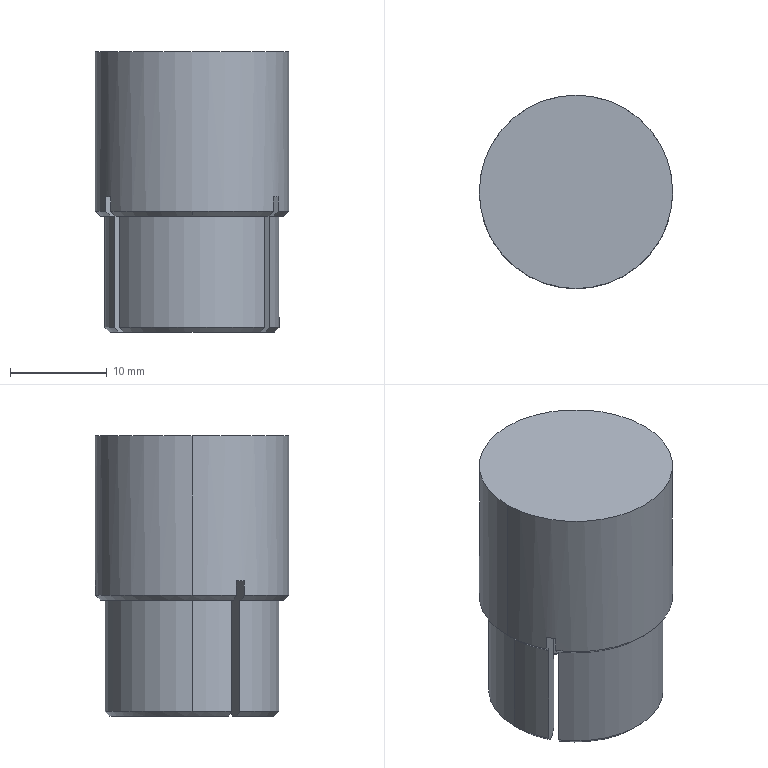Part | STEP file | BABR060_X2_8f9351658f74_X0_-14.STEP | 1 solid | 40 faces | box 20 x 20 x 29 mm | volume 3932 mm3 | plane 18 | cone 12 | cylinder 10 | commonest cylinder face diameters 18 x4 14 x2 15 x2 20 x2
STEP:
#1=CARTESIAN_POINT('',(-10.,0.,29.));
#2=VERTEX_POINT('',#1);
#3=CARTESIAN_POINT('',(10.,0.,29.));
#4=VERTEX_POINT('',#3);
#5=CARTESIAN_POINT('',(0.,0.,29.));
#6=DIRECTION('',(0.,0.,-1.));
#7=DIRECTION('',(-1.,0.,0.));
#8=AXIS2_PLACEMENT_3D('',#5,#6,#7);
#9=CIRCLE('',#8,10.);
#10=EDGE_CURVE('',#2,#4,#9,.T.);
#11=ORIENTED_EDGE('',*,*,#10,.T.);
#12=CARTESIAN_POINT('',(10.,0.,12.5));
#13=VERTEX_POINT('',#12);
#14=CARTESIAN_POINT('',(10.,0.,29.));
#15=DIRECTION('',(0.,0.,-1.));
#16=VECTOR('',#15,1000.);
#17=LINE('',#14,#16);
#18=EDGE_CURVE('',#4,#13,#17,.T.);
#19=ORIENTED_EDGE('',*,*,#18,.T.);
#20=CARTESIAN_POINT('',(0.5,9.987,12.5));
#21=VERTEX_POINT('',#20);
#22=CARTESIAN_POINT('',(0.,0.,12.5));
#23=DIRECTION('',(0.,0.,1.));
#24=DIRECTION('',(-1.,0.,0.));
#25=AXIS2_PLACEMENT_3D('',#22,#23,#24);
#26=CIRCLE('',#25,10.);
#27=EDGE_CURVE('',#13,#21,#26,.T.);
#28=ORIENTED_EDGE('',*,*,#27,.T.);
#29=CARTESIAN_POINT('',(0.5,9.987,14.));
#30=VERTEX_POINT('',#29);
#31=CARTESIAN_POINT('',(0.5,9.987,14.));
#32=DIRECTION('',(0.,0.,1.));
#33=VECTOR('',#32,1000.);
#34=LINE('',#31,#33);
#35=EDGE_CURVE('',#21,#30,#34,.T.);
#36=ORIENTED_EDGE('',*,*,#35,.T.);
#37=CARTESIAN_POINT('',(-0.5,9.987,14.));
#38=VERTEX_POINT('',#37);
#39=CARTESIAN_POINT('',(0.,0.,14.));
#40=DIRECTION('',(0.,0.,1.));
#41=DIRECTION('',(-1.,0.,0.));
#42=AXIS2_PLACEMENT_3D('',#39,#40,#41);
#43=CIRCLE('',#42,10.);
#44=EDGE_CURVE('',#30,#38,#43,.T.);
#45=ORIENTED_EDGE('',*,*,#44,.T.);
#46=CARTESIAN_POINT('',(-0.5,9.987,12.5));
#47=VERTEX_POINT('',#46);
#48=CARTESIAN_POINT('',(-0.5,9.987,14.));
#49=DIRECTION('',(0.,0.,-1.));
#50=VECTOR('',#49,1000.);
#51=LINE('',#48,#50);
#52=EDGE_CURVE('',#38,#47,#51,.T.);
#53=ORIENTED_EDGE('',*,*,#52,.T.);
#54=CARTESIAN_POINT('',(-10.,0.,12.5));
#55=VERTEX_POINT('',#54);
#56=CARTESIAN_POINT('',(0.,0.,12.5));
#57=DIRECTION('',(0.,0.,1.));
#58=DIRECTION('',(-1.,0.,0.));
#59=AXIS2_PLACEMENT_3D('',#56,#57,#58);
#60=CIRCLE('',#59,10.);
#61=EDGE_CURVE('',#47,#55,#60,.T.);
#62=ORIENTED_EDGE('',*,*,#61,.T.);
#63=CARTESIAN_POINT('',(-10.,0.,29.));
#64=DIRECTION('',(0.,0.,-1.));
#65=VECTOR('',#64,1000.);
#66=LINE('',#63,#65);
#67=EDGE_CURVE('',#2,#55,#66,.T.);
#68=ORIENTED_EDGE('',*,*,#67,.F.);
#69=EDGE_LOOP('',(#11,#19,#28,#36,#45,#53,#62,#68));
#70=FACE_OUTER_BOUND('',#69,.T.);
#71=CARTESIAN_POINT('',(0.,0.,29.));
#72=DIRECTION('',(0.,0.,-1.));
#73=DIRECTION('',(-1.,0.,0.));
#74=AXIS2_PLACEMENT_3D('',#71,#72,#73);
#75=CYLINDRICAL_SURFACE('',#74,10.);
#76=ADVANCED_FACE('',(#70),#75,.T.);
#77=CARTESIAN_POINT('',(-7.966,-5.176,12.));
#78=VERTEX_POINT('',#77);
#79=CARTESIAN_POINT('',(0.,-9.5,12.));
#80=VERTEX_POINT('',#79);
#81=CARTESIAN_POINT('',(0.,0.,12.));
#82=DIRECTION('',(0.,0.,1.));
#83=DIRECTION('',(0.,-1.,0.));
#84=AXIS2_PLACEMENT_3D('',#81,#82,#83);
#85=CIRCLE('',#84,9.5);
#86=EDGE_CURVE('',#78,#80,#85,.T.);
#87=ORIENTED_EDGE('',*,*,#86,.T.);
#88=CARTESIAN_POINT('',(0.,-10.,12.5));
#89=VERTEX_POINT('',#88);
#90=CARTESIAN_POINT('',(0.,-10.,12.5));
#91=DIRECTION('',(0.,-0.7071,0.7071));
#92=VECTOR('',#91,1000.);
#93=LINE('',#90,#92);
#94=EDGE_CURVE('',#80,#89,#93,.T.);
#95=ORIENTED_EDGE('',*,*,#94,.T.);
#96=CARTESIAN_POINT('',(-8.399,-5.427,12.5));
#97=VERTEX_POINT('',#96);
#98=CARTESIAN_POINT('',(0.,0.,12.5));
#99=DIRECTION('',(0.,0.,1.));
#100=DIRECTION('',(-1.,0.,0.));
#101=AXIS2_PLACEMENT_3D('',#98,#99,#100);
#102=CIRCLE('',#101,10.);
#103=EDGE_CURVE('',#97,#89,#102,.T.);
#104=ORIENTED_EDGE('',*,*,#103,.F.);
#105=CARTESIAN_POINT('',(-8.399,-5.427,12.5));
#106=CARTESIAN_POINT('',(-8.255,-5.343,12.333));
#107=CARTESIAN_POINT('',(-8.11,-5.26,12.167));
#108=CARTESIAN_POINT('',(-7.966,-5.176,12.));
#109=B_SPLINE_CURVE_WITH_KNOTS('',3,(#105,#106,#107,#108),.UNSPECIFIED.,.F.,.F.,(4,4),(0.,0.0007076),.UNSPECIFIED.);
#110=EDGE_CURVE('',#97,#78,#109,.T.);
#111=ORIENTED_EDGE('',*,*,#110,.T.);
#112=EDGE_LOOP('',(#87,#95,#104,#111));
#113=FACE_OUTER_BOUND('',#112,.T.);
#114=CARTESIAN_POINT('',(0.,0.,12.5));
#115=DIRECTION('',(0.,0.,1.));
#116=DIRECTION('',(0.,-1.,0.));
#117=AXIS2_PLACEMENT_3D('',#114,#115,#116);
#118=CONICAL_SURFACE('',#117,10.,0.7854);
#119=ADVANCED_FACE('',(#113),#118,.T.);
#120=CARTESIAN_POINT('',(-8.032,-4.06,12.));
#121=VERTEX_POINT('',#120);
#122=CARTESIAN_POINT('',(-9.,0.,12.));
#123=VERTEX_POINT('',#122);
#124=CARTESIAN_POINT('',(0.,0.,12.));
#125=DIRECTION('',(0.,0.,-1.));
#126=DIRECTION('',(-1.,0.,0.));
#127=AXIS2_PLACEMENT_3D('',#124,#125,#126);
#128=CIRCLE('',#127,9.);
#129=EDGE_CURVE('',#121,#123,#128,.T.);
#130=ORIENTED_EDGE('',*,*,#129,.T.);
#131=CARTESIAN_POINT('',(-9.,0.,0.5));
#132=VERTEX_POINT('',#131);
#133=CARTESIAN_POINT('',(-9.,0.,12.));
#134=DIRECTION('',(0.,0.,-1.));
#135=VECTOR('',#134,1000.);
#136=LINE('',#133,#135);
#137=EDGE_CURVE('',#123,#132,#136,.T.);
#138=ORIENTED_EDGE('',*,*,#137,.T.);
#139=CARTESIAN_POINT('',(-8.032,-4.06,0.5));
#140=VERTEX_POINT('',#139);
#141=CARTESIAN_POINT('',(0.,0.,0.5));
#142=DIRECTION('',(0.,0.,1.));
#143=DIRECTION('',(-1.,0.,0.));
#144=AXIS2_PLACEMENT_3D('',#141,#142,#143);
#145=CIRCLE('',#144,9.);
#146=EDGE_CURVE('',#132,#140,#145,.T.);
#147=ORIENTED_EDGE('',*,*,#146,.T.);
#148=CARTESIAN_POINT('',(-8.032,-4.06,12.));
#149=DIRECTION('',(0.,0.,1.));
#150=VECTOR('',#149,1000.);
#151=LINE('',#148,#150);
#152=EDGE_CURVE('',#140,#121,#151,.T.);
#153=ORIENTED_EDGE('',*,*,#152,.T.);
#154=EDGE_LOOP('',(#130,#138,#147,#153));
#155=FACE_OUTER_BOUND('',#154,.T.);
#156=CARTESIAN_POINT('',(0.,0.,12.));
#157=DIRECTION('',(0.,0.,-1.));
#158=DIRECTION('',(-1.,0.,0.));
#159=AXIS2_PLACEMENT_3D('',#156,#157,#158);
#160=CYLINDRICAL_SURFACE('',#159,9.);
#161=ADVANCED_FACE('',(#155),#160,.T.);
#162=CARTESIAN_POINT('',(7.598,-3.81,0.));
#163=VERTEX_POINT('',#162);
#164=CARTESIAN_POINT('',(8.5,0.,0.));
#165=VERTEX_POINT('',#164);
#166=CARTESIAN_POINT('',(0.,0.,0.));
#167=DIRECTION('',(0.,0.,1.));
#168=DIRECTION('',(1.,0.,0.));
#169=AXIS2_PLACEMENT_3D('',#166,#167,#168);
#170=CIRCLE('',#169,8.5);
#171=EDGE_CURVE('',#163,#165,#170,.T.);
#172=ORIENTED_EDGE('',*,*,#171,.T.);
#173=CARTESIAN_POINT('',(9.,0.,0.5));
#174=VERTEX_POINT('',#173);
#175=CARTESIAN_POINT('',(9.,0.,0.5));
#176=DIRECTION('',(0.7071,0.,0.7071));
#177=VECTOR('',#176,1000.);
#178=LINE('',#175,#177);
#179=EDGE_CURVE('',#165,#174,#178,.T.);
#180=ORIENTED_EDGE('',*,*,#179,.T.);
#181=CARTESIAN_POINT('',(8.032,-4.06,0.5));
#182=VERTEX_POINT('',#181);
#183=CARTESIAN_POINT('',(0.,0.,0.5));
#184=DIRECTION('',(0.,0.,1.));
#185=DIRECTION('',(-1.,0.,0.));
#186=AXIS2_PLACEMENT_3D('',#183,#184,#185);
#187=CIRCLE('',#186,9.);
#188=EDGE_CURVE('',#182,#174,#187,.T.);
#189=ORIENTED_EDGE('',*,*,#188,.F.);
#190=CARTESIAN_POINT('',(8.032,-4.06,0.5));
#191=CARTESIAN_POINT('',(7.888,-3.977,0.3333));
#192=CARTESIAN_POINT('',(7.743,-3.893,0.1667));
#193=CARTESIAN_POINT('',(7.598,-3.81,0.));
#194=B_SPLINE_CURVE_WITH_KNOTS('',3,(#190,#191,#192,#193),.UNSPECIFIED.,.F.,.F.,(4,4),(0.,0.0007077),.UNSPECIFIED.);
#195=EDGE_CURVE('',#182,#163,#194,.T.);
#196=ORIENTED_EDGE('',*,*,#195,.T.);
#197=EDGE_LOOP('',(#172,#180,#189,#196));
#198=FACE_OUTER_BOUND('',#197,.T.);
#199=CARTESIAN_POINT('',(0.,0.,0.5));
#200=DIRECTION('',(0.,0.,1.));
#201=DIRECTION('',(1.,0.,0.));
#202=AXIS2_PLACEMENT_3D('',#199,#200,#201);
#203=CONICAL_SURFACE('',#202,9.,0.7854);
#204=ADVANCED_FACE('',(#198),#203,.T.);
#205=CARTESIAN_POINT('',(7.,0.,14.5));
#206=VERTEX_POINT('',#205);
#207=CARTESIAN_POINT('',(-7.,0.,14.5));
#208=VERTEX_POINT('',#207);
#209=CARTESIAN_POINT('',(0.,0.,14.5));
#210=DIRECTION('',(0.,0.,-1.));
#211=DIRECTION('',(-1.,0.,0.));
#212=AXIS2_PLACEMENT_3D('',#209,#210,#211);
#213=CIRCLE('',#212,7.);
#214=EDGE_CURVE('',#206,#208,#213,.T.);
#215=ORIENTED_EDGE('',*,*,#214,.F.);
#216=CARTESIAN_POINT('',(7.,0.,0.5));
#217=VERTEX_POINT('',#216);
#218=CARTESIAN_POINT('',(7.,0.,14.5));
#219=DIRECTION('',(0.,0.,-1.));
#220=VECTOR('',#219,1000.);
#221=LINE('',#218,#220);
#222=EDGE_CURVE('',#206,#217,#221,.T.);
#223=ORIENTED_EDGE('',*,*,#222,.T.);
#224=CARTESIAN_POINT('',(6.297,-3.058,0.5));
#225=VERTEX_POINT('',#224);
#226=CARTESIAN_POINT('',(0.,0.,0.5));
#227=DIRECTION('',(0.,0.,1.));
#228=DIRECTION('',(-1.,0.,0.));
#229=AXIS2_PLACEMENT_3D('',#226,#227,#228);
#230=CIRCLE('',#229,7.);
#231=EDGE_CURVE('',#225,#217,#230,.T.);
#232=ORIENTED_EDGE('',*,*,#231,.F.);
#233=CARTESIAN_POINT('',(6.297,-3.058,14.));
#234=VERTEX_POINT('',#233);
#235=CARTESIAN_POINT('',(6.297,-3.058,14.));
#236=DIRECTION('',(0.,0.,1.));
#237=VECTOR('',#236,1000.);
#238=LINE('',#235,#237);
#239=EDGE_CURVE('',#225,#234,#238,.T.);
#240=ORIENTED_EDGE('',*,*,#239,.T.);
#241=CARTESIAN_POINT('',(5.797,-3.924,14.));
#242=VERTEX_POINT('',#241);
#243=CARTESIAN_POINT('',(0.,0.,14.));
#244=DIRECTION('',(0.,0.,1.));
#245=DIRECTION('',(-1.,0.,0.));
#246=AXIS2_PLACEMENT_3D('',#243,#244,#245);
#247=CIRCLE('',#246,7.);
#248=EDGE_CURVE('',#242,#234,#247,.T.);
#249=ORIENTED_EDGE('',*,*,#248,.F.);
#250=CARTESIAN_POINT('',(5.797,-3.924,0.5));
#251=VERTEX_POINT('',#250);
#252=CARTESIAN_POINT('',(5.797,-3.924,14.));
#253=DIRECTION('',(0.,0.,-1.));
#254=VECTOR('',#253,1000.);
#255=LINE('',#252,#254);
#256=EDGE_CURVE('',#242,#251,#255,.T.);
#257=ORIENTED_EDGE('',*,*,#256,.T.);
#258=CARTESIAN_POINT('',(-5.797,-3.924,0.5));
#259=VERTEX_POINT('',#258);
#260=CARTESIAN_POINT('',(0.,0.,0.5));
#261=DIRECTION('',(0.,0.,1.));
#262=DIRECTION('',(-1.,0.,0.));
#263=AXIS2_PLACEMENT_3D('',#260,#261,#262);
#264=CIRCLE('',#263,7.);
#265=EDGE_CURVE('',#259,#251,#264,.T.);
#266=ORIENTED_EDGE('',*,*,#265,.F.);
#267=CARTESIAN_POINT('',(-5.797,-3.924,14.));
#268=VERTEX_POINT('',#267);
#269=CARTESIAN_POINT('',(-5.797,-3.924,14.));
#270=DIRECTION('',(0.,0.,1.));
#271=VECTOR('',#270,1000.);
#272=LINE('',#269,#271);
#273=EDGE_CURVE('',#259,#268,#272,.T.);
#274=ORIENTED_EDGE('',*,*,#273,.T.);
#275=CARTESIAN_POINT('',(-6.297,-3.058,14.));
#276=VERTEX_POINT('',#275);
#277=CARTESIAN_POINT('',(0.,0.,14.));
#278=DIRECTION('',(0.,0.,-1.));
#279=DIRECTION('',(-1.,0.,0.));
#280=AXIS2_PLACEMENT_3D('',#277,#278,#279);
#281=CIRCLE('',#280,7.);
#282=EDGE_CURVE('',#268,#276,#281,.T.);
#283=ORIENTED_EDGE('',*,*,#282,.T.);
#284=CARTESIAN_POINT('',(-6.297,-3.058,0.5));
#285=VERTEX_POINT('',#284);
#286=CARTESIAN_POINT('',(-6.297,-3.058,14.));
#287=DIRECTION('',(0.,0.,-1.));
#288=VECTOR('',#287,1000.);
#289=LINE('',#286,#288);
#290=EDGE_CURVE('',#276,#285,#289,.T.);
#291=ORIENTED_EDGE('',*,*,#290,.T.);
#292=CARTESIAN_POINT('',(-7.,0.,0.5));
#293=VERTEX_POINT('',#292);
#294=CARTESIAN_POINT('',(0.,0.,0.5));
#295=DIRECTION('',(0.,0.,1.));
#296=DIRECTION('',(-1.,0.,0.));
#297=AXIS2_PLACEMENT_3D('',#294,#295,#296);
#298=CIRCLE('',#297,7.);
#299=EDGE_CURVE('',#293,#285,#298,.T.);
#300=ORIENTED_EDGE('',*,*,#299,.F.);
#301=CARTESIAN_POINT('',(-7.,0.,14.5));
#302=DIRECTION('',(0.,0.,-1.));
#303=VECTOR('',#302,1000.);
#304=LINE('',#301,#303);
#305=EDGE_CURVE('',#208,#293,#304,.T.);
#306=ORIENTED_EDGE('',*,*,#305,.F.);
#307=EDGE_LOOP('',(#215,#223,#232,#240,#249,#257,#266,#274,#283,#291,#300,#306));
#308=FACE_OUTER_BOUND('',#307,.T.);
#309=CARTESIAN_POINT('',(0.,0.,14.5));
#310=DIRECTION('',(0.,0.,-1.));
#311=DIRECTION('',(-1.,0.,0.));
#312=AXIS2_PLACEMENT_3D('',#309,#310,#311);
#313=CYLINDRICAL_SURFACE('',#312,7.);
#314=ADVANCED_FACE('',(#308),#313,.F.);
#315=CARTESIAN_POINT('',(-0.5,6.982,0.5));
#316=VERTEX_POINT('',#315);
#317=CARTESIAN_POINT('',(0.,0.,0.5));
#318=DIRECTION('',(0.,0.,1.));
#319=DIRECTION('',(-1.,0.,0.));
#320=AXIS2_PLACEMENT_3D('',#317,#318,#319);
#321=CIRCLE('',#320,7.);
#322=EDGE_CURVE('',#316,#293,#321,.T.);
#323=ORIENTED_EDGE('',*,*,#322,.T.);
#324=CARTESIAN_POINT('',(-7.5,0.,0.));
#325=VERTEX_POINT('',#324);
#326=CARTESIAN_POINT('',(-7.5,0.,0.));
#327=DIRECTION('',(-0.7071,0.,-0.7071));
#328=VECTOR('',#327,1000.);
#329=LINE('',#326,#328);
#330=EDGE_CURVE('',#293,#325,#329,.T.);
#331=ORIENTED_EDGE('',*,*,#330,.T.);
#332=CARTESIAN_POINT('',(-0.5,7.483,0.));
#333=VERTEX_POINT('',#332);
#334=CARTESIAN_POINT('',(0.,0.,0.));
#335=DIRECTION('',(0.,0.,-1.));
#336=DIRECTION('',(-1.,0.,0.));
#337=AXIS2_PLACEMENT_3D('',#334,#335,#336);
#338=CIRCLE('',#337,7.5);
#339=EDGE_CURVE('',#325,#333,#338,.T.);
#340=ORIENTED_EDGE('',*,*,#339,.T.);
#341=CARTESIAN_POINT('',(-0.5,6.982,0.5));
#342=CARTESIAN_POINT('',(-0.5,7.149,0.3333));
#343=CARTESIAN_POINT('',(-0.5,7.316,0.1667));
#344=CARTESIAN_POINT('',(-0.5,7.483,0.));
#345=B_SPLINE_CURVE_WITH_KNOTS('',3,(#341,#342,#343,#344),.UNSPECIFIED.,.F.,.F.,(4,4),(0.,0.000708),.UNSPECIFIED.);
#346=EDGE_CURVE('',#316,#333,#345,.T.);
#347=ORIENTED_EDGE('',*,*,#346,.F.);
#348=EDGE_LOOP('',(#323,#331,#340,#347));
#349=FACE_OUTER_BOUND('',#348,.T.);
#350=CARTESIAN_POINT('',(0.,0.,0.));
#351=DIRECTION('',(0.,0.,-1.));
#352=DIRECTION('',(-1.,0.,0.));
#353=AXIS2_PLACEMENT_3D('',#350,#351,#352);
#354=CONICAL_SURFACE('',#353,7.5,0.7854);
#355=ADVANCED_FACE('',(#349),#354,.F.);
#356=CARTESIAN_POINT('',(7.5,0.,26.5));
#357=VERTEX_POINT('',#356);
#358=CARTESIAN_POINT('',(-7.5,0.,26.5));
#359=VERTEX_POINT('',#358);
#360=CARTESIAN_POINT('',(0.,0.,26.5));
#361=DIRECTION('',(0.,0.,-1.));
#362=DIRECTION('',(-1.,0.,0.));
#363=AXIS2_PLACEMENT_3D('',#360,#361,#362);
#364=CIRCLE('',#363,7.5);
#365=EDGE_CURVE('',#357,#359,#364,.T.);
#366=ORIENTED_EDGE('',*,*,#365,.F.);
#367=CARTESIAN_POINT('',(7.5,0.,14.5));
#368=VERTEX_POINT('',#367);
#369=CARTESIAN_POINT('',(7.5,0.,26.5));
#370=DIRECTION('',(0.,0.,-1.));
#371=VECTOR('',#370,1000.);
#372=LINE('',#369,#371);
#373=EDGE_CURVE('',#357,#368,#372,.T.);
#374=ORIENTED_EDGE('',*,*,#373,.T.);
#375=CARTESIAN_POINT('',(-7.5,0.,14.5));
#376=VERTEX_POINT('',#375);
#377=CARTESIAN_POINT('',(0.,0.,14.5));
#378=DIRECTION('',(0.,0.,-1.));
#379=DIRECTION('',(-1.,0.,0.));
#380=AXIS2_PLACEMENT_3D('',#377,#378,#379);
#381=CIRCLE('',#380,7.5);
#382=EDGE_CURVE('',#368,#376,#381,.T.);
#383=ORIENTED_EDGE('',*,*,#382,.T.);
#384=CARTESIAN_POINT('',(-7.5,0.,26.5));
#385=DIRECTION('',(0.,0.,-1.));
#386=VECTOR('',#385,1000.);
#387=LINE('',#384,#386);
#388=EDGE_CURVE('',#359,#376,#387,.T.);
#389=ORIENTED_EDGE('',*,*,#388,.F.);
#390=EDGE_LOOP('',(#366,#374,#383,#389));
#391=FACE_OUTER_BOUND('',#390,.T.);
#392=CARTESIAN_POINT('',(0.,0.,26.5));
#393=DIRECTION('',(0.,0.,-1.));
#394=DIRECTION('',(-1.,0.,0.));
#395=AXIS2_PLACEMENT_3D('',#392,#393,#394);
#396=CYLINDRICAL_SURFACE('',#395,7.5);
#397=ADVANCED_FACE('',(#391),#396,.F.);
#398=ORIENTED_EDGE('',*,*,#18,.F.);
#399=CARTESIAN_POINT('',(0.,0.,29.));
#400=DIRECTION('',(0.,0.,-1.));
#401=DIRECTION('',(-1.,0.,0.));
#402=AXIS2_PLACEMENT_3D('',#399,#400,#401);
#403=CIRCLE('',#402,10.);
#404=EDGE_CURVE('',#4,#2,#403,.T.);
#405=ORIENTED_EDGE('',*,*,#404,.T.);
#406=ORIENTED_EDGE('',*,*,#67,.T.);
#407=CARTESIAN_POINT('',(-8.899,-4.561,12.5));
#408=VERTEX_POINT('',#407);
#409=CARTESIAN_POINT('',(0.,0.,12.5));
#410=DIRECTION('',(0.,0.,1.));
#411=DIRECTION('',(-1.,0.,0.));
#412=AXIS2_PLACEMENT_3D('',#409,#410,#411);
#413=CIRCLE('',#412,10.);
#414=EDGE_CURVE('',#55,#408,#413,.T.);
#415=ORIENTED_EDGE('',*,*,#414,.T.);
#416=CARTESIAN_POINT('',(-8.899,-4.561,14.));
#417=VERTEX_POINT('',#416);
#418=CARTESIAN_POINT('',(-8.899,-4.561,14.));
#419=DIRECTION('',(0.,0.,1.));
#420=VECTOR('',#419,1000.);
#421=LINE('',#418,#420);
#422=EDGE_CURVE('',#408,#417,#421,.T.);
#423=ORIENTED_EDGE('',*,*,#422,.T.);
#424=CARTESIAN_POINT('',(-8.399,-5.427,14.));
#425=VERTEX_POINT('',#424);
#426=CARTESIAN_POINT('',(0.,0.,14.));
#427=DIRECTION('',(0.,0.,1.));
#428=DIRECTION('',(-1.,0.,0.));
#429=AXIS2_PLACEMENT_3D('',#426,#427,#428);
#430=CIRCLE('',#429,10.);
#431=EDGE_CURVE('',#417,#425,#430,.T.);
#432=ORIENTED_EDGE('',*,*,#431,.T.);
#433=CARTESIAN_POINT('',(-8.399,-5.427,14.));
#434=DIRECTION('',(0.,0.,-1.));
#435=VECTOR('',#434,1000.);
#436=LINE('',#433,#435);
#437=EDGE_CURVE('',#425,#97,#436,.T.);
#438=ORIENTED_EDGE('',*,*,#437,.T.);
#439=ORIENTED_EDGE('',*,*,#103,.T.);
#440=CARTESIAN_POINT('',(8.399,-5.427,12.5));
#441=VERTEX_POINT('',#440);
#442=CARTESIAN_POINT('',(0.,0.,12.5));
#443=DIRECTION('',(0.,0.,1.));
#444=DIRECTION('',(-1.,0.,0.));
#445=AXIS2_PLACEMENT_3D('',#442,#443,#444);
#446=CIRCLE('',#445,10.);
#447=EDGE_CURVE('',#89,#441,#446,.T.);
#448=ORIENTED_EDGE('',*,*,#447,.T.);
#449=CARTESIAN_POINT('',(8.399,-5.427,14.));
#450=VERTEX_POINT('',#449);
#451=CARTESIAN_POINT('',(8.399,-5.427,14.));
#452=DIRECTION('',(0.,0.,1.));
#453=VECTOR('',#452,1000.);
#454=LINE('',#451,#453);
#455=EDGE_CURVE('',#441,#450,#454,.T.);
#456=ORIENTED_EDGE('',*,*,#455,.T.);
#457=CARTESIAN_POINT('',(8.899,-4.561,14.));
#458=VERTEX_POINT('',#457);
#459=CARTESIAN_POINT('',(0.,0.,14.));
#460=DIRECTION('',(0.,0.,1.));
#461=DIRECTION('',(-1.,0.,0.));
#462=AXIS2_PLACEMENT_3D('',#459,#460,#461);
#463=CIRCLE('',#462,10.);
#464=EDGE_CURVE('',#450,#458,#463,.T.);
#465=ORIENTED_EDGE('',*,*,#464,.T.);
#466=CARTESIAN_POINT('',(8.899,-4.561,12.5));
#467=VERTEX_POINT('',#466);
#468=CARTESIAN_POINT('',(8.899,-4.561,14.));
#469=DIRECTION('',(0.,0.,-1.));
#470=VECTOR('',#469,1000.);
#471=LINE('',#468,#470);
#472=EDGE_CURVE('',#458,#467,#471,.T.);
#473=ORIENTED_EDGE('',*,*,#472,.T.);
#474=CARTESIAN_POINT('',(0.,0.,12.5));
#475=DIRECTION('',(0.,0.,1.));
#476=DIRECTION('',(-1.,0.,0.));
#477=AXIS2_PLACEMENT_3D('',#474,#475,#476);
#478=CIRCLE('',#477,10.);
#479=EDGE_CURVE('',#467,#13,#478,.T.);
#480=ORIENTED_EDGE('',*,*,#479,.T.);
#481=EDGE_LOOP('',(#398,#405,#406,#415,#423,#432,#438,#439,#448,#456,#465,#473,#480));
#482=FACE_OUTER_BOUND('',#481,.T.);
#483=CARTESIAN_POINT('',(0.,0.,29.));
#484=DIRECTION('',(0.,0.,-1.));
#485=DIRECTION('',(-1.,0.,0.));
#486=AXIS2_PLACEMENT_3D('',#483,#484,#485);
#487=CYLINDRICAL_SURFACE('',#486,10.);
#488=ADVANCED_FACE('',(#482),#487,.T.);
#489=CARTESIAN_POINT('',(-0.5,9.487,12.));
#490=VERTEX_POINT('',#489);
#491=CARTESIAN_POINT('',(-0.5,9.987,12.5));
#492=CARTESIAN_POINT('',(-0.5,9.821,12.333));
#493=CARTESIAN_POINT('',(-0.5,9.654,12.167));
#494=CARTESIAN_POINT('',(-0.5,9.487,12.));
#495=B_SPLINE_CURVE_WITH_KNOTS('',3,(#491,#492,#493,#494),.UNSPECIFIED.,.F.,.F.,(4,4),(0.,0.0007076),.UNSPECIFIED.);
#496=EDGE_CURVE('',#47,#490,#495,.T.);
#497=ORIENTED_EDGE('',*,*,#496,.T.);
#498=CARTESIAN_POINT('',(-8.466,-4.31,12.));
#499=VERTEX_POINT('',#498);
#500=CARTESIAN_POINT('',(0.,0.,12.));
#501=DIRECTION('',(0.,0.,1.));
#502=DIRECTION('',(0.,-1.,0.));
#503=AXIS2_PLACEMENT_3D('',#500,#501,#502);
#504=CIRCLE('',#503,9.5);
#505=EDGE_CURVE('',#490,#499,#504,.T.);
#506=ORIENTED_EDGE('',*,*,#505,.T.);
#507=CARTESIAN_POINT('',(-8.466,-4.31,12.));
#508=CARTESIAN_POINT('',(-8.61,-4.394,12.167));
#509=CARTESIAN_POINT('',(-8.755,-4.477,12.333));
#510=CARTESIAN_POINT('',(-8.899,-4.561,12.5));
#511=B_SPLINE_CURVE_WITH_KNOTS('',3,(#507,#508,#509,#510),.UNSPECIFIED.,.F.,.F.,(4,4),(0.,0.0007076),.UNSPECIFIED.);
#512=EDGE_CURVE('',#499,#408,#511,.T.);
#513=ORIENTED_EDGE('',*,*,#512,.T.);
#514=ORIENTED_EDGE('',*,*,#414,.F.);
#515=ORIENTED_EDGE('',*,*,#61,.F.);
#516=EDGE_LOOP('',(#497,#506,#513,#514,#515));
#517=FACE_OUTER_BOUND('',#516,.T.);
#518=CARTESIAN_POINT('',(0.,0.,12.5));
#519=DIRECTION('',(0.,0.,1.));
#520=DIRECTION('',(0.,-1.,0.));
#521=AXIS2_PLACEMENT_3D('',#518,#519,#520);
#522=CONICAL_SURFACE('',#521,10.,0.7854);
#523=ADVANCED_FACE('',(#517),#522,.T.);
#524=CARTESIAN_POINT('',(0.5,9.487,12.));
#525=VERTEX_POINT('',#524);
#526=CARTESIAN_POINT('',(0.5,9.487,12.));
#527=CARTESIAN_POINT('',(0.5,9.654,12.167));
#528=CARTESIAN_POINT('',(0.5,9.821,12.333));
#529=CARTESIAN_POINT('',(0.5,9.987,12.5));
#530=B_SPLINE_CURVE_WITH_KNOTS('',3,(#526,#527,#528,#529),.UNSPECIFIED.,.F.,.F.,(4,4),(0.,0.0007076),.UNSPECIFIED.);
#531=EDGE_CURVE('',#525,#21,#530,.T.);
#532=ORIENTED_EDGE('',*,*,#531,.T.);
#533=ORIENTED_EDGE('',*,*,#27,.F.);
#534=ORIENTED_EDGE('',*,*,#479,.F.);
#535=CARTESIAN_POINT('',(8.466,-4.31,12.));
#536=VERTEX_POINT('',#535);
#537=CARTESIAN_POINT('',(8.899,-4.561,12.5));
#538=CARTESIAN_POINT('',(8.755,-4.477,12.333));
#539=CARTESIAN_POINT('',(8.61,-4.394,12.167));
#540=CARTESIAN_POINT('',(8.466,-4.31,12.));
#541=B_SPLINE_CURVE_WITH_KNOTS('',3,(#537,#538,#539,#540),.UNSPECIFIED.,.F.,.F.,(4,4),(0.,0.0007076),.UNSPECIFIED.);
#542=EDGE_CURVE('',#467,#536,#541,.T.);
#543=ORIENTED_EDGE('',*,*,#542,.T.);
#544=CARTESIAN_POINT('',(0.,0.,12.));
#545=DIRECTION('',(0.,0.,1.));
#546=DIRECTION('',(0.,-1.,0.));
#547=AXIS2_PLACEMENT_3D('',#544,#545,#546);
#548=CIRCLE('',#547,9.5);
#549=EDGE_CURVE('',#536,#525,#548,.T.);
#550=ORIENTED_EDGE('',*,*,#549,.T.);
#551=EDGE_LOOP('',(#532,#533,#534,#543,#550));
#552=FACE_OUTER_BOUND('',#551,.T.);
#553=CARTESIAN_POINT('',(0.,0.,12.5));
#554=DIRECTION('',(0.,0.,1.));
#555=DIRECTION('',(0.,-1.,0.));
#556=AXIS2_PLACEMENT_3D('',#553,#554,#555);
#557=CONICAL_SURFACE('',#556,10.,0.7854);
#558=ADVANCED_FACE('',(#552),#557,.T.);
#559=ORIENTED_EDGE('',*,*,#10,.F.);
#560=ORIENTED_EDGE('',*,*,#404,.F.);
#561=EDGE_LOOP('',(#559,#560));
#562=FACE_OUTER_BOUND('',#561,.T.);
#563=CARTESIAN_POINT('',(0.,0.,29.));
#564=DIRECTION('',(0.,0.,1.));
#565=DIRECTION('',(1.,0.,0.));
#566=AXIS2_PLACEMENT_3D('',#563,#564,#565);
#567=PLANE('',#566);
#568=ADVANCED_FACE('',(#562),#567,.T.);
#569=ORIENTED_EDGE('',*,*,#94,.F.);
#570=CARTESIAN_POINT('',(7.966,-5.176,12.));
#571=VERTEX_POINT('',#570);
#572=CARTESIAN_POINT('',(0.,0.,12.));
#573=DIRECTION('',(0.,0.,1.));
#574=DIRECTION('',(0.,-1.,0.));
#575=AXIS2_PLACEMENT_3D('',#572,#573,#574);
#576=CIRCLE('',#575,9.5);
#577=EDGE_CURVE('',#80,#571,#576,.T.);
#578=ORIENTED_EDGE('',*,*,#577,.T.);
#579=CARTESIAN_POINT('',(7.966,-5.176,12.));
#580=CARTESIAN_POINT('',(8.11,-5.26,12.167));
#581=CARTESIAN_POINT('',(8.255,-5.343,12.333));
#582=CARTESIAN_POINT('',(8.399,-5.427,12.5));
#583=B_SPLINE_CURVE_WITH_KNOTS('',3,(#579,#580,#581,#582),.UNSPECIFIED.,.F.,.F.,(4,4),(0.,0.0007076),.UNSPECIFIED.);
#584=EDGE_CURVE('',#571,#441,#583,.T.);
#585=ORIENTED_EDGE('',*,*,#584,.T.);
#586=ORIENTED_EDGE('',*,*,#447,.F.);
#587=EDGE_LOOP('',(#569,#578,#585,#586));
#588=FACE_OUTER_BOUND('',#587,.T.);
#589=CARTESIAN_POINT('',(0.,0.,12.5));
#590=DIRECTION('',(0.,0.,1.));
#591=DIRECTION('',(0.,-1.,0.));
#592=AXIS2_PLACEMENT_3D('',#589,#590,#591);
#593=CONICAL_SURFACE('',#592,10.,0.7854);
#594=ADVANCED_FACE('',(#588),#593,.T.);
#595=ORIENTED_EDGE('',*,*,#129,.F.);
#596=CARTESIAN_POINT('',(-5.212,-2.432,12.));
#597=DIRECTION('',(-0.866,-0.5,0.));
#598=VECTOR('',#597,1000.);
#599=LINE('',#596,#598);
#600=EDGE_CURVE('',#121,#499,#599,.T.);
#601=ORIENTED_EDGE('',*,*,#600,.T.);
#602=ORIENTED_EDGE('',*,*,#505,.F.);
#603=CARTESIAN_POINT('',(-0.5,8.986,12.));
#604=VERTEX_POINT('',#603);
#605=CARTESIAN_POINT('',(-0.5,10.505,12.));
#606=DIRECTION('',(0.,-1.,0.));
#607=VECTOR('',#606,1000.);
#608=LINE('',#605,#607);
#609=EDGE_CURVE('',#490,#604,#608,.T.);
#610=ORIENTED_EDGE('',*,*,#609,.T.);
#611=CARTESIAN_POINT('',(0.,0.,12.));
#612=DIRECTION('',(0.,0.,-1.));
#613=DIRECTION('',(-1.,0.,0.));
#614=AXIS2_PLACEMENT_3D('',#611,#612,#613);
#615=CIRCLE('',#614,9.);
#616=EDGE_CURVE('',#123,#604,#615,.T.);
#617=ORIENTED_EDGE('',*,*,#616,.F.);
#618=EDGE_LOOP('',(#595,#601,#602,#610,#617));
#619=FACE_OUTER_BOUND('',#618,.T.);
#620=CARTESIAN_POINT('',(0.,0.,12.));
#621=DIRECTION('',(0.,0.,1.));
#622=DIRECTION('',(1.,0.,0.));
#623=AXIS2_PLACEMENT_3D('',#620,#621,#622);
#624=PLANE('',#623);
#625=ADVANCED_FACE('',(#619),#624,.F.);
#626=CARTESIAN_POINT('',(0.5,8.986,12.));
#627=VERTEX_POINT('',#626);
#628=CARTESIAN_POINT('',(0.5,5.73,12.));
#629=DIRECTION('',(0.,1.,0.));
#630=VECTOR('',#629,1000.);
#631=LINE('',#628,#630);
#632=EDGE_CURVE('',#627,#525,#631,.T.);
#633=ORIENTED_EDGE('',*,*,#632,.T.);
#634=ORIENTED_EDGE('',*,*,#549,.F.);
#635=CARTESIAN_POINT('',(8.032,-4.06,12.));
#636=VERTEX_POINT('',#635);
#637=CARTESIAN_POINT('',(9.348,-4.82,12.));
#638=DIRECTION('',(-0.866,0.5,0.));
#639=VECTOR('',#638,1000.);
#640=LINE('',#637,#639);
#641=EDGE_CURVE('',#536,#636,#640,.T.);
#642=ORIENTED_EDGE('',*,*,#641,.T.);
#643=CARTESIAN_POINT('',(0.,0.,12.));
#644=DIRECTION('',(0.,0.,-1.));
#645=DIRECTION('',(-1.,0.,0.));
#646=AXIS2_PLACEMENT_3D('',#643,#644,#645);
#647=CIRCLE('',#646,9.);
#648=EDGE_CURVE('',#627,#636,#647,.T.);
#649=ORIENTED_EDGE('',*,*,#648,.F.);
#650=EDGE_LOOP('',(#633,#634,#642,#649));
#651=FACE_OUTER_BOUND('',#650,.T.);
#652=CARTESIAN_POINT('',(0.,0.,12.));
#653=DIRECTION('',(0.,0.,1.));
#654=DIRECTION('',(1.,0.,0.));
#655=AXIS2_PLACEMENT_3D('',#652,#653,#654);
#656=PLANE('',#655);
#657=ADVANCED_FACE('',(#651),#656,.F.);
#658=CARTESIAN_POINT('',(-7.532,-4.926,12.));
#659=VERTEX_POINT('',#658);
#660=CARTESIAN_POINT('',(-8.848,-5.686,12.));
#661=DIRECTION('',(0.866,0.5,0.));
#662=VECTOR('',#661,1000.);
#663=LINE('',#660,#662);
#664=EDGE_CURVE('',#78,#659,#663,.T.);
#665=ORIENTED_EDGE('',*,*,#664,.T.);
#666=CARTESIAN_POINT('',(7.532,-4.926,12.));
#667=VERTEX_POINT('',#666);
#668=CARTESIAN_POINT('',(0.,0.,12.));
#669=DIRECTION('',(0.,0.,-1.));
#670=DIRECTION('',(-1.,0.,0.));
#671=AXIS2_PLACEMENT_3D('',#668,#669,#670);
#672=CIRCLE('',#671,9.);
#673=EDGE_CURVE('',#667,#659,#672,.T.);
#674=ORIENTED_EDGE('',*,*,#673,.F.);
#675=CARTESIAN_POINT('',(4.712,-3.298,12.));
#676=DIRECTION('',(0.866,-0.5,0.));
#677=VECTOR('',#676,1000.);
#678=LINE('',#675,#677);
#679=EDGE_CURVE('',#667,#571,#678,.T.);
#680=ORIENTED_EDGE('',*,*,#679,.T.);
#681=ORIENTED_EDGE('',*,*,#577,.F.);
#682=ORIENTED_EDGE('',*,*,#86,.F.);
#683=EDGE_LOOP('',(#665,#674,#680,#681,#682));
#684=FACE_OUTER_BOUND('',#683,.T.);
#685=CARTESIAN_POINT('',(0.,0.,12.));
#686=DIRECTION('',(0.,0.,1.));
#687=DIRECTION('',(1.,0.,0.));
#688=AXIS2_PLACEMENT_3D('',#685,#686,#687);
#689=PLANE('',#688);
#690=ADVANCED_FACE('',(#684),#689,.F.);
#691=ORIENTED_EDGE('',*,*,#137,.F.);
#692=ORIENTED_EDGE('',*,*,#616,.T.);
#693=CARTESIAN_POINT('',(-0.5,8.986,0.5));
#694=VERTEX_POINT('',#693);
#695=CARTESIAN_POINT('',(-0.5,8.986,12.));
#696=DIRECTION('',(0.,0.,-1.));
#697=VECTOR('',#696,1000.);
#698=LINE('',#695,#697);
#699=EDGE_CURVE('',#604,#694,#698,.T.);
#700=ORIENTED_EDGE('',*,*,#699,.T.);
#701=CARTESIAN_POINT('',(0.,0.,0.5));
#702=DIRECTION('',(0.,0.,1.));
#703=DIRECTION('',(-1.,0.,0.));
#704=AXIS2_PLACEMENT_3D('',#701,#702,#703);
#705=CIRCLE('',#704,9.);
#706=EDGE_CURVE('',#694,#132,#705,.T.);
#707=ORIENTED_EDGE('',*,*,#706,.T.);
#708=EDGE_LOOP('',(#691,#692,#700,#707));
#709=FACE_OUTER_BOUND('',#708,.T.);
#710=CARTESIAN_POINT('',(0.,0.,12.));
#711=DIRECTION('',(0.,0.,-1.));
#712=DIRECTION('',(-1.,0.,0.));
#713=AXIS2_PLACEMENT_3D('',#710,#711,#712);
#714=CYLINDRICAL_SURFACE('',#713,9.);
#715=ADVANCED_FACE('',(#709),#714,.T.);
#716=ORIENTED_EDGE('',*,*,#648,.T.);
#717=CARTESIAN_POINT('',(8.032,-4.06,12.));
#718=DIRECTION('',(0.,0.,-1.));
#719=VECTOR('',#718,1000.);
#720=LINE('',#717,#719);
#721=EDGE_CURVE('',#636,#182,#720,.T.);
#722=ORIENTED_EDGE('',*,*,#721,.T.);
#723=ORIENTED_EDGE('',*,*,#188,.T.);
#724=CARTESIAN_POINT('',(0.5,8.986,0.5));
#725=VERTEX_POINT('',#724);
#726=CARTESIAN_POINT('',(0.,0.,0.5));
#727=DIRECTION('',(0.,0.,1.));
#728=DIRECTION('',(-1.,0.,0.));
#729=AXIS2_PLACEMENT_3D('',#726,#727,#728);
#730=CIRCLE('',#729,9.);
#731=EDGE_CURVE('',#174,#725,#730,.T.);
#732=ORIENTED_EDGE('',*,*,#731,.T.);
#733=CARTESIAN_POINT('',(0.5,8.986,12.));
#734=DIRECTION('',(0.,0.,1.));
#735=VECTOR('',#734,1000.);
#736=LINE('',#733,#735);
#737=EDGE_CURVE('',#725,#627,#736,.T.);
#738=ORIENTED_EDGE('',*,*,#737,.T.);
#739=EDGE_LOOP('',(#716,#722,#723,#732,#738));
#740=FACE_OUTER_BOUND('',#739,.T.);
#741=CARTESIAN_POINT('',(0.,0.,12.));
#742=DIRECTION('',(0.,0.,-1.));
#743=DIRECTION('',(-1.,0.,0.));
#744=AXIS2_PLACEMENT_3D('',#741,#742,#743);
#745=CYLINDRICAL_SURFACE('',#744,9.);
#746=ADVANCED_FACE('',(#740),#745,.T.);
#747=CARTESIAN_POINT('',(-7.532,-4.926,0.5));
#748=VERTEX_POINT('',#747);
#749=CARTESIAN_POINT('',(7.532,-4.926,0.5));
#750=VERTEX_POINT('',#749);
#751=CARTESIAN_POINT('',(0.,0.,0.5));
#752=DIRECTION('',(0.,0.,1.));
#753=DIRECTION('',(-1.,0.,0.));
#754=AXIS2_PLACEMENT_3D('',#751,#752,#753);
#755=CIRCLE('',#754,9.);
#756=EDGE_CURVE('',#748,#750,#755,.T.);
#757=ORIENTED_EDGE('',*,*,#756,.T.);
#758=CARTESIAN_POINT('',(7.532,-4.926,12.));
#759=DIRECTION('',(0.,0.,1.));
#760=VECTOR('',#759,1000.);
#761=LINE('',#758,#760);
#762=EDGE_CURVE('',#750,#667,#761,.T.);
#763=ORIENTED_EDGE('',*,*,#762,.T.);
#764=ORIENTED_EDGE('',*,*,#673,.T.);
#765=CARTESIAN_POINT('',(-7.532,-4.926,12.));
#766=DIRECTION('',(0.,0.,-1.));
#767=VECTOR('',#766,1000.);
#768=LINE('',#765,#767);
#769=EDGE_CURVE('',#659,#748,#768,.T.);
#770=ORIENTED_EDGE('',*,*,#769,.T.);
#771=EDGE_LOOP('',(#757,#763,#764,#770));
#772=FACE_OUTER_BOUND('',#771,.T.);
#773=CARTESIAN_POINT('',(0.,0.,12.));
#774=DIRECTION('',(0.,0.,-1.));
#775=DIRECTION('',(-1.,0.,0.));
#776=AXIS2_PLACEMENT_3D('',#773,#774,#775);
#777=CYLINDRICAL_SURFACE('',#776,9.);
#778=ADVANCED_FACE('',(#772),#777,.T.);
#779=CARTESIAN_POINT('',(-0.5,8.485,0.));
#780=VERTEX_POINT('',#779);
#781=CARTESIAN_POINT('',(-0.5,8.986,0.5));
#782=CARTESIAN_POINT('',(-0.5,8.819,0.3333));
#783=CARTESIAN_POINT('',(-0.5,8.652,0.1667));
#784=CARTESIAN_POINT('',(-0.5,8.485,0.));
#785=B_SPLINE_CURVE_WITH_KNOTS('',3,(#781,#782,#783,#784),.UNSPECIFIED.,.F.,.F.,(4,4),(0.,0.0007077),.UNSPECIFIED.);
#786=EDGE_CURVE('',#694,#780,#785,.T.);
#787=ORIENTED_EDGE('',*,*,#786,.T.);
#788=CARTESIAN_POINT('',(-7.598,-3.81,0.));
#789=VERTEX_POINT('',#788);
#790=CARTESIAN_POINT('',(0.,0.,0.));
#791=DIRECTION('',(0.,0.,1.));
#792=DIRECTION('',(1.,0.,0.));
#793=AXIS2_PLACEMENT_3D('',#790,#791,#792);
#794=CIRCLE('',#793,8.5);
#795=EDGE_CURVE('',#780,#789,#794,.T.);
#796=ORIENTED_EDGE('',*,*,#795,.T.);
#797=CARTESIAN_POINT('',(-7.598,-3.81,0.));
#798=CARTESIAN_POINT('',(-7.743,-3.893,0.1667));
#799=CARTESIAN_POINT('',(-7.888,-3.977,0.3333));
#800=CARTESIAN_POINT('',(-8.032,-4.06,0.5));
#801=B_SPLINE_CURVE_WITH_KNOTS('',3,(#797,#798,#799,#800),.UNSPECIFIED.,.F.,.F.,(4,4),(0.,0.0007077),.UNSPECIFIED.);
#802=EDGE_CURVE('',#789,#140,#801,.T.);
#803=ORIENTED_EDGE('',*,*,#802,.T.);
#804=ORIENTED_EDGE('',*,*,#146,.F.);
#805=ORIENTED_EDGE('',*,*,#706,.F.);
#806=EDGE_LOOP('',(#787,#796,#803,#804,#805));
#807=FACE_OUTER_BOUND('',#806,.T.);
#808=CARTESIAN_POINT('',(0.,0.,0.5));
#809=DIRECTION('',(0.,0.,1.));
#810=DIRECTION('',(1.,0.,0.));
#811=AXIS2_PLACEMENT_3D('',#808,#809,#810);
#812=CONICAL_SURFACE('',#811,9.,0.7854);
#813=ADVANCED_FACE('',(#807),#812,.T.);
#814=CARTESIAN_POINT('',(-0.5,10.505,0.));
#815=DIRECTION('',(0.,-1.,0.));
#816=VECTOR('',#815,1000.);
#817=LINE('',#814,#816);
#818=EDGE_CURVE('',#780,#333,#817,.T.);
#819=ORIENTED_EDGE('',*,*,#818,.F.);
#820=ORIENTED_EDGE('',*,*,#786,.F.);
#821=ORIENTED_EDGE('',*,*,#699,.F.);
#822=ORIENTED_EDGE('',*,*,#609,.F.);
#823=ORIENTED_EDGE('',*,*,#496,.F.);
#824=ORIENTED_EDGE('',*,*,#52,.F.);
#825=CARTESIAN_POINT('',(-0.5,6.982,14.));
#826=VERTEX_POINT('',#825);
#827=CARTESIAN_POINT('',(-0.5,10.505,14.));
#828=DIRECTION('',(0.,1.,0.));
#829=VECTOR('',#828,1000.);
#830=LINE('',#827,#829);
#831=EDGE_CURVE('',#826,#38,#830,.T.);
#832=ORIENTED_EDGE('',*,*,#831,.F.);
#833=CARTESIAN_POINT('',(-0.5,6.982,14.));
#834=DIRECTION('',(0.,0.,1.));
#835=VECTOR('',#834,1000.);
#836=LINE('',#833,#835);
#837=EDGE_CURVE('',#316,#826,#836,.T.);
#838=ORIENTED_EDGE('',*,*,#837,.F.);
#839=ORIENTED_EDGE('',*,*,#346,.T.);
#840=EDGE_LOOP('',(#819,#820,#821,#822,#823,#824,#832,#838,#839));
#841=FACE_OUTER_BOUND('',#840,.T.);
#842=CARTESIAN_POINT('',(-0.5,10.505,14.));
#843=DIRECTION('',(-1.,0.,0.));
#844=DIRECTION('',(0.,-1.,0.));
#845=AXIS2_PLACEMENT_3D('',#842,#843,#844);
#846=PLANE('',#845);
#847=ADVANCED_FACE('',(#841),#846,.F.);
#848=ORIENTED_EDGE('',*,*,#422,.F.);
#849=ORIENTED_EDGE('',*,*,#512,.F.);
#850=ORIENTED_EDGE('',*,*,#600,.F.);
#851=ORIENTED_EDGE('',*,*,#152,.F.);
#852=ORIENTED_EDGE('',*,*,#802,.F.);
#853=CARTESIAN_POINT('',(-6.731,-3.309,0.));
#854=VERTEX_POINT('',#853);
#855=CARTESIAN_POINT('',(-5.212,-2.432,0.));
#856=DIRECTION('',(-0.866,-0.5,0.));
#857=VECTOR('',#856,1000.);
#858=LINE('',#855,#857);
#859=EDGE_CURVE('',#854,#789,#858,.T.);
#860=ORIENTED_EDGE('',*,*,#859,.F.);
#861=CARTESIAN_POINT('',(-6.731,-3.309,0.));
#862=CARTESIAN_POINT('',(-6.586,-3.225,0.1667));
#863=CARTESIAN_POINT('',(-6.441,-3.142,0.3333));
#864=CARTESIAN_POINT('',(-6.297,-3.058,0.5));
#865=B_SPLINE_CURVE_WITH_KNOTS('',3,(#861,#862,#863,#864),.UNSPECIFIED.,.F.,.F.,(4,4),(0.,0.000708),.UNSPECIFIED.);
#866=EDGE_CURVE('',#854,#285,#865,.T.);
#867=ORIENTED_EDGE('',*,*,#866,.T.);
#868=ORIENTED_EDGE('',*,*,#290,.F.);
#869=CARTESIAN_POINT('',(-5.212,-2.432,14.));
#870=DIRECTION('',(0.866,0.5,0.));
#871=VECTOR('',#870,1000.);
#872=LINE('',#869,#871);
#873=EDGE_CURVE('',#417,#276,#872,.T.);
#874=ORIENTED_EDGE('',*,*,#873,.F.);
#875=EDGE_LOOP('',(#848,#849,#850,#851,#852,#860,#867,#868,#874));
#876=FACE_OUTER_BOUND('',#875,.T.);
#877=CARTESIAN_POINT('',(-5.212,-2.432,14.));
#878=DIRECTION('',(-0.5,0.866,0.));
#879=DIRECTION('',(-0.866,-0.5,0.));
#880=AXIS2_PLACEMENT_3D('',#877,#878,#879);
#881=PLANE('',#880);
#882=ADVANCED_FACE('',(#876),#881,.F.);
#883=CARTESIAN_POINT('',(6.731,-3.309,0.));
#884=VERTEX_POINT('',#883);
#885=CARTESIAN_POINT('',(6.731,-3.309,0.));
#886=DIRECTION('',(0.866,-0.5,0.));
#887=VECTOR('',#886,1000.);
#888=LINE('',#885,#887);
#889=EDGE_CURVE('',#884,#163,#888,.T.);
#890=ORIENTED_EDGE('',*,*,#889,.T.);
#891=ORIENTED_EDGE('',*,*,#195,.F.);
#892=ORIENTED_EDGE('',*,*,#721,.F.);
#893=ORIENTED_EDGE('',*,*,#641,.F.);
#894=ORIENTED_EDGE('',*,*,#542,.F.);
#895=ORIENTED_EDGE('',*,*,#472,.F.);
#896=CARTESIAN_POINT('',(9.348,-4.82,14.));
#897=DIRECTION('',(0.866,-0.5,0.));
#898=VECTOR('',#897,1000.);
#899=LINE('',#896,#898);
#900=EDGE_CURVE('',#234,#458,#899,.T.);
#901=ORIENTED_EDGE('',*,*,#900,.F.);
#902=ORIENTED_EDGE('',*,*,#239,.F.);
#903=CARTESIAN_POINT('',(6.297,-3.058,0.5));
#904=CARTESIAN_POINT('',(6.441,-3.142,0.3333));
#905=CARTESIAN_POINT('',(6.586,-3.225,0.1667));
#906=CARTESIAN_POINT('',(6.731,-3.309,0.));
#907=B_SPLINE_CURVE_WITH_KNOTS('',3,(#903,#904,#905,#906),.UNSPECIFIED.,.F.,.F.,(4,4),(0.,0.000708),.UNSPECIFIED.);
#908=EDGE_CURVE('',#225,#884,#907,.T.);
#909=ORIENTED_EDGE('',*,*,#908,.T.);
#910=EDGE_LOOP('',(#890,#891,#892,#893,#894,#895,#901,#902,#909));
#911=FACE_OUTER_BOUND('',#910,.T.);
#912=CARTESIAN_POINT('',(9.348,-4.82,14.));
#913=DIRECTION('',(0.5,0.866,0.));
#914=DIRECTION('',(-0.866,0.5,0.));
#915=AXIS2_PLACEMENT_3D('',#912,#913,#914);
#916=PLANE('',#915);
#917=ADVANCED_FACE('',(#911),#916,.F.);
#918=ORIENTED_EDGE('',*,*,#35,.F.);
#919=ORIENTED_EDGE('',*,*,#531,.F.);
#920=ORIENTED_EDGE('',*,*,#632,.F.);
#921=ORIENTED_EDGE('',*,*,#737,.F.);
#922=CARTESIAN_POINT('',(0.5,8.485,0.));
#923=VERTEX_POINT('',#922);
#924=CARTESIAN_POINT('',(0.5,8.485,0.));
#925=CARTESIAN_POINT('',(0.5,8.652,0.1667));
#926=CARTESIAN_POINT('',(0.5,8.819,0.3333));
#927=CARTESIAN_POINT('',(0.5,8.986,0.5));
#928=B_SPLINE_CURVE_WITH_KNOTS('',3,(#924,#925,#926,#927),.UNSPECIFIED.,.F.,.F.,(4,4),(0.,0.0007077),.UNSPECIFIED.);
#929=EDGE_CURVE('',#923,#725,#928,.T.);
#930=ORIENTED_EDGE('',*,*,#929,.F.);
#931=CARTESIAN_POINT('',(0.5,7.483,0.));
#932=VERTEX_POINT('',#931);
#933=CARTESIAN_POINT('',(0.5,0.,0.));
#934=DIRECTION('',(0.,-1.,0.));
#935=VECTOR('',#934,1000.);
#936=LINE('',#933,#935);
#937=EDGE_CURVE('',#923,#932,#936,.T.);
#938=ORIENTED_EDGE('',*,*,#937,.T.);
#939=CARTESIAN_POINT('',(0.5,6.982,0.5));
#940=VERTEX_POINT('',#939);
#941=CARTESIAN_POINT('',(0.5,7.483,0.));
#942=CARTESIAN_POINT('',(0.5,7.316,0.1667));
#943=CARTESIAN_POINT('',(0.5,7.149,0.3333));
#944=CARTESIAN_POINT('',(0.5,6.982,0.5));
#945=B_SPLINE_CURVE_WITH_KNOTS('',3,(#941,#942,#943,#944),.UNSPECIFIED.,.F.,.F.,(4,4),(0.,0.000708),.UNSPECIFIED.);
#946=EDGE_CURVE('',#932,#940,#945,.T.);
#947=ORIENTED_EDGE('',*,*,#946,.T.);
#948=CARTESIAN_POINT('',(0.5,6.982,14.));
#949=VERTEX_POINT('',#948);
#950=CARTESIAN_POINT('',(0.5,6.982,14.));
#951=DIRECTION('',(0.,0.,-1.));
#952=VECTOR('',#951,1000.);
#953=LINE('',#950,#952);
#954=EDGE_CURVE('',#949,#940,#953,.T.);
#955=ORIENTED_EDGE('',*,*,#954,.F.);
#956=CARTESIAN_POINT('',(0.5,5.73,14.));
#957=DIRECTION('',(0.,-1.,0.));
#958=VECTOR('',#957,1000.);
#959=LINE('',#956,#958);
#960=EDGE_CURVE('',#30,#949,#959,.T.);
#961=ORIENTED_EDGE('',*,*,#960,.F.);
#962=EDGE_LOOP('',(#918,#919,#920,#921,#930,#938,#947,#955,#961));
#963=FACE_OUTER_BOUND('',#962,.T.);
#964=CARTESIAN_POINT('',(0.5,5.73,14.));
#965=DIRECTION('',(1.,0.,0.));
#966=DIRECTION('',(0.,1.,0.));
#967=AXIS2_PLACEMENT_3D('',#964,#965,#966);
#968=PLANE('',#967);
#969=ADVANCED_FACE('',(#963),#968,.F.);
#970=ORIENTED_EDGE('',*,*,#179,.F.);
#971=CARTESIAN_POINT('',(0.,0.,0.));
#972=DIRECTION('',(0.,0.,1.));
#973=DIRECTION('',(1.,0.,0.));
#974=AXIS2_PLACEMENT_3D('',#971,#972,#973);
#975=CIRCLE('',#974,8.5);
#976=EDGE_CURVE('',#165,#923,#975,.T.);
#977=ORIENTED_EDGE('',*,*,#976,.T.);
#978=ORIENTED_EDGE('',*,*,#929,.T.);
#979=ORIENTED_EDGE('',*,*,#731,.F.);
#980=EDGE_LOOP('',(#970,#977,#978,#979));
#981=FACE_OUTER_BOUND('',#980,.T.);
#982=CARTESIAN_POINT('',(0.,0.,0.5));
#983=DIRECTION('',(0.,0.,1.));
#984=DIRECTION('',(1.,0.,0.));
#985=AXIS2_PLACEMENT_3D('',#982,#983,#984);
#986=CONICAL_SURFACE('',#985,9.,0.7854);
#987=ADVANCED_FACE('',(#981),#986,.T.);
#988=ORIENTED_EDGE('',*,*,#455,.F.);
#989=ORIENTED_EDGE('',*,*,#584,.F.);
#990=ORIENTED_EDGE('',*,*,#679,.F.);
#991=ORIENTED_EDGE('',*,*,#762,.F.);
#992=CARTESIAN_POINT('',(7.098,-4.676,0.));
#993=VERTEX_POINT('',#992);
#994=CARTESIAN_POINT('',(7.098,-4.676,0.));
#995=CARTESIAN_POINT('',(7.243,-4.759,0.1667));
#996=CARTESIAN_POINT('',(7.388,-4.843,0.3333));
#997=CARTESIAN_POINT('',(7.532,-4.926,0.5));
#998=B_SPLINE_CURVE_WITH_KNOTS('',3,(#994,#995,#996,#997),.UNSPECIFIED.,.F.,.F.,(4,4),(0.,0.0007077),.UNSPECIFIED.);
#999=EDGE_CURVE('',#993,#750,#998,.T.);
#1000=ORIENTED_EDGE('',*,*,#999,.F.);
#1001=CARTESIAN_POINT('',(6.231,-4.175,0.));
#1002=VERTEX_POINT('',#1001);
#1003=CARTESIAN_POINT('',(7.098,-4.676,0.));
#1004=DIRECTION('',(-0.866,0.5,0.));
#1005=VECTOR('',#1004,1000.);
#1006=LINE('',#1003,#1005);
#1007=EDGE_CURVE('',#993,#1002,#1006,.T.);
#1008=ORIENTED_EDGE('',*,*,#1007,.T.);
#1009=CARTESIAN_POINT('',(6.231,-4.175,0.));
#1010=CARTESIAN_POINT('',(6.086,-4.091,0.1667));
#1011=CARTESIAN_POINT('',(5.941,-4.008,0.3333));
#1012=CARTESIAN_POINT('',(5.797,-3.924,0.5));
#1013=B_SPLINE_CURVE_WITH_KNOTS('',3,(#1009,#1010,#1011,#1012),.UNSPECIFIED.,.F.,.F.,(4,4),(0.,0.000708),.UNSPECIFIED.);
#1014=EDGE_CURVE('',#1002,#251,#1013,.T.);
#1015=ORIENTED_EDGE('',*,*,#1014,.T.);
#1016=ORIENTED_EDGE('',*,*,#256,.F.);
#1017=CARTESIAN_POINT('',(4.712,-3.298,14.));
#1018=DIRECTION('',(-0.866,0.5,0.));
#1019=VECTOR('',#1018,1000.);
#1020=LINE('',#1017,#1019);
#1021=EDGE_CURVE('',#450,#242,#1020,.T.);
#1022=ORIENTED_EDGE('',*,*,#1021,.F.);
#1023=EDGE_LOOP('',(#988,#989,#990,#991,#1000,#1008,#1015,#1016,#1022));
#1024=FACE_OUTER_BOUND('',#1023,.T.);
#1025=CARTESIAN_POINT('',(4.712,-3.298,14.));
#1026=DIRECTION('',(-0.5,-0.866,0.));
#1027=DIRECTION('',(0.866,-0.5,0.));
#1028=AXIS2_PLACEMENT_3D('',#1025,#1026,#1027);
#1029=PLANE('',#1028);
#1030=ADVANCED_FACE('',(#1024),#1029,.F.);
#1031=ORIENTED_EDGE('',*,*,#999,.T.);
#1032=ORIENTED_EDGE('',*,*,#756,.F.);
#1033=CARTESIAN_POINT('',(-7.098,-4.676,0.));
#1034=VERTEX_POINT('',#1033);
#1035=CARTESIAN_POINT('',(-7.532,-4.926,0.5));
#1036=CARTESIAN_POINT('',(-7.388,-4.843,0.3333));
#1037=CARTESIAN_POINT('',(-7.243,-4.759,0.1667));
#1038=CARTESIAN_POINT('',(-7.098,-4.676,0.));
#1039=B_SPLINE_CURVE_WITH_KNOTS('',3,(#1035,#1036,#1037,#1038),.UNSPECIFIED.,.F.,.F.,(4,4),(0.,0.0007077),.UNSPECIFIED.);
#1040=EDGE_CURVE('',#748,#1034,#1039,.T.);
#1041=ORIENTED_EDGE('',*,*,#1040,.T.);
#1042=CARTESIAN_POINT('',(0.,0.,0.));
#1043=DIRECTION('',(0.,0.,1.));
#1044=DIRECTION('',(1.,0.,0.));
#1045=AXIS2_PLACEMENT_3D('',#1042,#1043,#1044);
#1046=CIRCLE('',#1045,8.5);
#1047=EDGE_CURVE('',#1034,#993,#1046,.T.);
#1048=ORIENTED_EDGE('',*,*,#1047,.T.);
#1049=EDGE_LOOP('',(#1031,#1032,#1041,#1048));
#1050=FACE_OUTER_BOUND('',#1049,.T.);
#1051=CARTESIAN_POINT('',(0.,0.,0.5));
#1052=DIRECTION('',(0.,0.,1.));
#1053=DIRECTION('',(1.,0.,0.));
#1054=AXIS2_PLACEMENT_3D('',#1051,#1052,#1053);
#1055=CONICAL_SURFACE('',#1054,9.,0.7854);
#1056=ADVANCED_FACE('',(#1050),#1055,.T.);
#1057=CARTESIAN_POINT('',(-6.231,-4.175,0.));
#1058=VERTEX_POINT('',#1057);
#1059=CARTESIAN_POINT('',(-8.848,-5.686,0.));
#1060=DIRECTION('',(0.866,0.5,0.));
#1061=VECTOR('',#1060,1000.);
#1062=LINE('',#1059,#1061);
#1063=EDGE_CURVE('',#1034,#1058,#1062,.T.);
#1064=ORIENTED_EDGE('',*,*,#1063,.F.);
#1065=ORIENTED_EDGE('',*,*,#1040,.F.);
#1066=ORIENTED_EDGE('',*,*,#769,.F.);
#1067=ORIENTED_EDGE('',*,*,#664,.F.);
#1068=ORIENTED_EDGE('',*,*,#110,.F.);
#1069=ORIENTED_EDGE('',*,*,#437,.F.);
#1070=CARTESIAN_POINT('',(-8.848,-5.686,14.));
#1071=DIRECTION('',(-0.866,-0.5,0.));
#1072=VECTOR('',#1071,1000.);
#1073=LINE('',#1070,#1072);
#1074=EDGE_CURVE('',#268,#425,#1073,.T.);
#1075=ORIENTED_EDGE('',*,*,#1074,.F.);
#1076=ORIENTED_EDGE('',*,*,#273,.F.);
#1077=CARTESIAN_POINT('',(-5.797,-3.924,0.5));
#1078=CARTESIAN_POINT('',(-5.941,-4.008,0.3333));
#1079=CARTESIAN_POINT('',(-6.086,-4.091,0.1667));
#1080=CARTESIAN_POINT('',(-6.231,-4.175,0.));
#1081=B_SPLINE_CURVE_WITH_KNOTS('',3,(#1077,#1078,#1079,#1080),.UNSPECIFIED.,.F.,.F.,(4,4),(0.,0.000708),.UNSPECIFIED.);
#1082=EDGE_CURVE('',#259,#1058,#1081,.T.);
#1083=ORIENTED_EDGE('',*,*,#1082,.T.);
#1084=EDGE_LOOP('',(#1064,#1065,#1066,#1067,#1068,#1069,#1075,#1076,#1083));
#1085=FACE_OUTER_BOUND('',#1084,.T.);
#1086=CARTESIAN_POINT('',(-8.848,-5.686,14.));
#1087=DIRECTION('',(0.5,-0.866,0.));
#1088=DIRECTION('',(0.866,0.5,0.));
#1089=AXIS2_PLACEMENT_3D('',#1086,#1087,#1088);
#1090=PLANE('',#1089);
#1091=ADVANCED_FACE('',(#1085),#1090,.F.);
#1092=CARTESIAN_POINT('',(0.,0.,0.));
#1093=DIRECTION('',(0.,0.,-1.));
#1094=DIRECTION('',(-1.,0.,0.));
#1095=AXIS2_PLACEMENT_3D('',#1092,#1093,#1094);
#1096=CIRCLE('',#1095,7.5);
#1097=EDGE_CURVE('',#854,#325,#1096,.T.);
#1098=ORIENTED_EDGE('',*,*,#1097,.F.);
#1099=ORIENTED_EDGE('',*,*,#859,.T.);
#1100=ORIENTED_EDGE('',*,*,#795,.F.);
#1101=ORIENTED_EDGE('',*,*,#818,.T.);
#1102=ORIENTED_EDGE('',*,*,#339,.F.);
#1103=EDGE_LOOP('',(#1098,#1099,#1100,#1101,#1102));
#1104=FACE_OUTER_BOUND('',#1103,.T.);
#1105=CARTESIAN_POINT('',(0.,0.,0.));
#1106=DIRECTION('',(0.,0.,1.));
#1107=DIRECTION('',(1.,0.,0.));
#1108=AXIS2_PLACEMENT_3D('',#1105,#1106,#1107);
#1109=PLANE('',#1108);
#1110=ADVANCED_FACE('',(#1104),#1109,.F.);
#1111=CARTESIAN_POINT('',(0.,0.,14.));
#1112=DIRECTION('',(0.,0.,-1.));
#1113=DIRECTION('',(-1.,0.,0.));
#1114=AXIS2_PLACEMENT_3D('',#1111,#1112,#1113);
#1115=CIRCLE('',#1114,7.);
#1116=EDGE_CURVE('',#826,#949,#1115,.T.);
#1117=ORIENTED_EDGE('',*,*,#1116,.F.);
#1118=ORIENTED_EDGE('',*,*,#831,.T.);
#1119=ORIENTED_EDGE('',*,*,#44,.F.);
#1120=ORIENTED_EDGE('',*,*,#960,.T.);
#1121=EDGE_LOOP('',(#1117,#1118,#1119,#1120));
#1122=FACE_OUTER_BOUND('',#1121,.T.);
#1123=CARTESIAN_POINT('',(0.,0.,14.));
#1124=DIRECTION('',(0.,0.,1.));
#1125=DIRECTION('',(1.,0.,0.));
#1126=AXIS2_PLACEMENT_3D('',#1123,#1124,#1125);
#1127=PLANE('',#1126);
#1128=ADVANCED_FACE('',(#1122),#1127,.F.);
#1129=ORIENTED_EDGE('',*,*,#222,.F.);
#1130=CARTESIAN_POINT('',(0.,0.,14.5));
#1131=DIRECTION('',(0.,0.,-1.));
#1132=DIRECTION('',(-1.,0.,0.));
#1133=AXIS2_PLACEMENT_3D('',#1130,#1131,#1132);
#1134=CIRCLE('',#1133,7.);
#1135=EDGE_CURVE('',#208,#206,#1134,.T.);
#1136=ORIENTED_EDGE('',*,*,#1135,.F.);
#1137=ORIENTED_EDGE('',*,*,#305,.T.);
#1138=ORIENTED_EDGE('',*,*,#322,.F.);
#1139=ORIENTED_EDGE('',*,*,#837,.T.);
#1140=ORIENTED_EDGE('',*,*,#1116,.T.);
#1141=ORIENTED_EDGE('',*,*,#954,.T.);
#1142=CARTESIAN_POINT('',(0.,0.,0.5));
#1143=DIRECTION('',(0.,0.,1.));
#1144=DIRECTION('',(-1.,0.,0.));
#1145=AXIS2_PLACEMENT_3D('',#1142,#1143,#1144);
#1146=CIRCLE('',#1145,7.);
#1147=EDGE_CURVE('',#217,#940,#1146,.T.);
#1148=ORIENTED_EDGE('',*,*,#1147,.F.);
#1149=EDGE_LOOP('',(#1129,#1136,#1137,#1138,#1139,#1140,#1141,#1148));
#1150=FACE_OUTER_BOUND('',#1149,.T.);
#1151=CARTESIAN_POINT('',(0.,0.,14.5));
#1152=DIRECTION('',(0.,0.,-1.));
#1153=DIRECTION('',(-1.,0.,0.));
#1154=AXIS2_PLACEMENT_3D('',#1151,#1152,#1153);
#1155=CYLINDRICAL_SURFACE('',#1154,7.);
#1156=ADVANCED_FACE('',(#1150),#1155,.F.);
#1157=ORIENTED_EDGE('',*,*,#282,.F.);
#1158=ORIENTED_EDGE('',*,*,#1074,.T.);
#1159=ORIENTED_EDGE('',*,*,#431,.F.);
#1160=ORIENTED_EDGE('',*,*,#873,.T.);
#1161=EDGE_LOOP('',(#1157,#1158,#1159,#1160));
#1162=FACE_OUTER_BOUND('',#1161,.T.);
#1163=CARTESIAN_POINT('',(0.,0.,14.));
#1164=DIRECTION('',(0.,0.,1.));
#1165=DIRECTION('',(1.,0.,0.));
#1166=AXIS2_PLACEMENT_3D('',#1163,#1164,#1165);
#1167=PLANE('',#1166);
#1168=ADVANCED_FACE('',(#1162),#1167,.F.);
#1169=ORIENTED_EDGE('',*,*,#248,.T.);
#1170=ORIENTED_EDGE('',*,*,#900,.T.);
#1171=ORIENTED_EDGE('',*,*,#464,.F.);
#1172=ORIENTED_EDGE('',*,*,#1021,.T.);
#1173=EDGE_LOOP('',(#1169,#1170,#1171,#1172));
#1174=FACE_OUTER_BOUND('',#1173,.T.);
#1175=CARTESIAN_POINT('',(0.,0.,14.));
#1176=DIRECTION('',(0.,0.,1.));
#1177=DIRECTION('',(1.,0.,0.));
#1178=AXIS2_PLACEMENT_3D('',#1175,#1176,#1177);
#1179=PLANE('',#1178);
#1180=ADVANCED_FACE('',(#1174),#1179,.F.);
#1181=ORIENTED_EDGE('',*,*,#937,.F.);
#1182=ORIENTED_EDGE('',*,*,#976,.F.);
#1183=ORIENTED_EDGE('',*,*,#171,.F.);
#1184=ORIENTED_EDGE('',*,*,#889,.F.);
#1185=CARTESIAN_POINT('',(0.,0.,0.));
#1186=DIRECTION('',(0.,0.,-1.));
#1187=DIRECTION('',(-1.,0.,0.));
#1188=AXIS2_PLACEMENT_3D('',#1185,#1186,#1187);
#1189=CIRCLE('',#1188,7.5);
#1190=EDGE_CURVE('',#932,#884,#1189,.T.);
#1191=ORIENTED_EDGE('',*,*,#1190,.F.);
#1192=EDGE_LOOP('',(#1181,#1182,#1183,#1184,#1191));
#1193=FACE_OUTER_BOUND('',#1192,.T.);
#1194=CARTESIAN_POINT('',(0.,0.,0.));
#1195=DIRECTION('',(0.,0.,1.));
#1196=DIRECTION('',(1.,0.,0.));
#1197=AXIS2_PLACEMENT_3D('',#1194,#1195,#1196);
#1198=PLANE('',#1197);
#1199=ADVANCED_FACE('',(#1193),#1198,.F.);
#1200=ORIENTED_EDGE('',*,*,#1063,.T.);
#1201=CARTESIAN_POINT('',(0.,0.,0.));
#1202=DIRECTION('',(0.,0.,-1.));
#1203=DIRECTION('',(-1.,0.,0.));
#1204=AXIS2_PLACEMENT_3D('',#1201,#1202,#1203);
#1205=CIRCLE('',#1204,7.5);
#1206=EDGE_CURVE('',#1002,#1058,#1205,.T.);
#1207=ORIENTED_EDGE('',*,*,#1206,.F.);
#1208=ORIENTED_EDGE('',*,*,#1007,.F.);
#1209=ORIENTED_EDGE('',*,*,#1047,.F.);
#1210=EDGE_LOOP('',(#1200,#1207,#1208,#1209));
#1211=FACE_OUTER_BOUND('',#1210,.T.);
#1212=CARTESIAN_POINT('',(0.,0.,0.));
#1213=DIRECTION('',(0.,0.,1.));
#1214=DIRECTION('',(1.,0.,0.));
#1215=AXIS2_PLACEMENT_3D('',#1212,#1213,#1214);
#1216=PLANE('',#1215);
#1217=ADVANCED_FACE('',(#1211),#1216,.F.);
#1218=ORIENTED_EDGE('',*,*,#330,.F.);
#1219=ORIENTED_EDGE('',*,*,#299,.T.);
#1220=ORIENTED_EDGE('',*,*,#866,.F.);
#1221=ORIENTED_EDGE('',*,*,#1097,.T.);
#1222=EDGE_LOOP('',(#1218,#1219,#1220,#1221));
#1223=FACE_OUTER_BOUND('',#1222,.T.);
#1224=CARTESIAN_POINT('',(0.,0.,0.));
#1225=DIRECTION('',(0.,0.,-1.));
#1226=DIRECTION('',(-1.,0.,0.));
#1227=AXIS2_PLACEMENT_3D('',#1224,#1225,#1226);
#1228=CONICAL_SURFACE('',#1227,7.5,0.7854);
#1229=ADVANCED_FACE('',(#1223),#1228,.F.);
#1230=CARTESIAN_POINT('',(0.,0.,14.5));
#1231=DIRECTION('',(0.,0.,-1.));
#1232=DIRECTION('',(-1.,0.,0.));
#1233=AXIS2_PLACEMENT_3D('',#1230,#1231,#1232);
#1234=CIRCLE('',#1233,7.5);
#1235=EDGE_CURVE('',#376,#368,#1234,.T.);
#1236=ORIENTED_EDGE('',*,*,#1235,.F.);
#1237=ORIENTED_EDGE('',*,*,#382,.F.);
#1238=EDGE_LOOP('',(#1236,#1237));
#1239=FACE_OUTER_BOUND('',#1238,.T.);
#1240=ORIENTED_EDGE('',*,*,#1135,.T.);
#1241=ORIENTED_EDGE('',*,*,#214,.T.);
#1242=EDGE_LOOP('',(#1240,#1241));
#1243=FACE_BOUND('',#1242,.T.);
#1244=CARTESIAN_POINT('',(0.,0.,14.5));
#1245=DIRECTION('',(0.,0.,-1.));
#1246=DIRECTION('',(-1.,0.,0.));
#1247=AXIS2_PLACEMENT_3D('',#1244,#1245,#1246);
#1248=PLANE('',#1247);
#1249=ADVANCED_FACE('',(#1239,#1243),#1248,.F.);
#1250=ORIENTED_EDGE('',*,*,#1190,.T.);
#1251=ORIENTED_EDGE('',*,*,#908,.F.);
#1252=ORIENTED_EDGE('',*,*,#231,.T.);
#1253=ORIENTED_EDGE('',*,*,#1147,.T.);
#1254=ORIENTED_EDGE('',*,*,#946,.F.);
#1255=EDGE_LOOP('',(#1250,#1251,#1252,#1253,#1254));
#1256=FACE_OUTER_BOUND('',#1255,.T.);
#1257=CARTESIAN_POINT('',(0.,0.,0.));
#1258=DIRECTION('',(0.,0.,-1.));
#1259=DIRECTION('',(-1.,0.,0.));
#1260=AXIS2_PLACEMENT_3D('',#1257,#1258,#1259);
#1261=CONICAL_SURFACE('',#1260,7.5,0.7854);
#1262=ADVANCED_FACE('',(#1256),#1261,.F.);
#1263=ORIENTED_EDGE('',*,*,#265,.T.);
#1264=ORIENTED_EDGE('',*,*,#1014,.F.);
#1265=ORIENTED_EDGE('',*,*,#1206,.T.);
#1266=ORIENTED_EDGE('',*,*,#1082,.F.);
#1267=EDGE_LOOP('',(#1263,#1264,#1265,#1266));
#1268=FACE_OUTER_BOUND('',#1267,.T.);
#1269=CARTESIAN_POINT('',(0.,0.,0.));
#1270=DIRECTION('',(0.,0.,-1.));
#1271=DIRECTION('',(-1.,0.,0.));
#1272=AXIS2_PLACEMENT_3D('',#1269,#1270,#1271);
#1273=CONICAL_SURFACE('',#1272,7.5,0.7854);
#1274=ADVANCED_FACE('',(#1268),#1273,.F.);
#1275=ORIENTED_EDGE('',*,*,#373,.F.);
#1276=CARTESIAN_POINT('',(0.,0.,26.5));
#1277=DIRECTION('',(0.,0.,-1.));
#1278=DIRECTION('',(-1.,0.,0.));
#1279=AXIS2_PLACEMENT_3D('',#1276,#1277,#1278);
#1280=CIRCLE('',#1279,7.5);
#1281=EDGE_CURVE('',#359,#357,#1280,.T.);
#1282=ORIENTED_EDGE('',*,*,#1281,.F.);
#1283=ORIENTED_EDGE('',*,*,#388,.T.);
#1284=ORIENTED_EDGE('',*,*,#1235,.T.);
#1285=EDGE_LOOP('',(#1275,#1282,#1283,#1284));
#1286=FACE_OUTER_BOUND('',#1285,.T.);
#1287=CARTESIAN_POINT('',(0.,0.,26.5));
#1288=DIRECTION('',(0.,0.,-1.));
#1289=DIRECTION('',(-1.,0.,0.));
#1290=AXIS2_PLACEMENT_3D('',#1287,#1288,#1289);
#1291=CYLINDRICAL_SURFACE('',#1290,7.5);
#1292=ADVANCED_FACE('',(#1286),#1291,.F.);
#1293=ORIENTED_EDGE('',*,*,#1281,.T.);
#1294=ORIENTED_EDGE('',*,*,#365,.T.);
#1295=EDGE_LOOP('',(#1293,#1294));
#1296=FACE_OUTER_BOUND('',#1295,.T.);
#1297=CARTESIAN_POINT('',(0.,0.,26.5));
#1298=DIRECTION('',(0.,0.,-1.));
#1299=DIRECTION('',(-1.,0.,0.));
#1300=AXIS2_PLACEMENT_3D('',#1297,#1298,#1299);
#1301=PLANE('',#1300);
#1302=ADVANCED_FACE('',(#1296),#1301,.T.);
#1303=CLOSED_SHELL('',(#76,#119,#161,#204,#314,#355,#397,#488,#523,#558,#568,#594,#625,#657,#690,#715,#746,#778,#813,#847,#882,#917,#969,#987,#1030,#1056,#1091,#1110,#1128,#1156,#1168,#1180,#1199,#1217,#1229,#1249,#1262,#1274,#1292,#1302));
#1304=MANIFOLD_SOLID_BREP('',#1303);
#1305=CARTESIAN_POINT('',(0.,0.,0.));
#1306=DIRECTION('',(0.,0.,1.));
#1307=DIRECTION('',(1.,0.,0.));
#1308=AXIS2_PLACEMENT_3D('',#1305,#1306,#1307);
#1309=(LENGTH_UNIT()NAMED_UNIT(*)SI_UNIT(.MILLI.,.METRE.));
#1310=UNCERTAINTY_MEASURE_WITH_UNIT(LENGTH_MEASURE(0.00001),#1309,'','');
#1311=(NAMED_UNIT(*)PLANE_ANGLE_UNIT()SI_UNIT($,.RADIAN.));
#1312=(NAMED_UNIT(*)SI_UNIT($,.STERADIAN.)SOLID_ANGLE_UNIT());
#1313=(GEOMETRIC_REPRESENTATION_CONTEXT(3)GLOBAL_UNCERTAINTY_ASSIGNED_CONTEXT((#1310))GLOBAL_UNIT_ASSIGNED_CONTEXT((#1309,#1311,#1312))REPRESENTATION_CONTEXT('',''));
#1314=ADVANCED_BREP_SHAPE_REPRESENTATION('',(#1304,#1308),#1313);